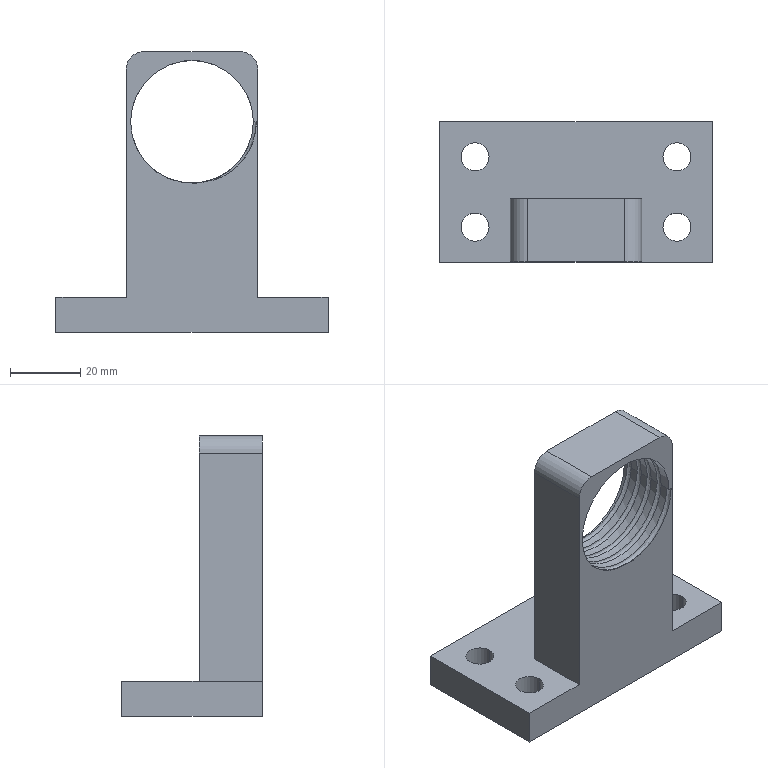Part | NX | features SKETCH 3, DATUM_CSYS 2, BREP 1, DATUM_ON_PATH 1, EXTRUDE 1, HELIX 1, VARIATIONAL_SWEEP 1 | 1 solid | 33 faces | volume 58227 mm3 | cylinder 21 | plane 11 | spline 1 | commonest cylinder face diameters 35 x11 8 x8 10 x2